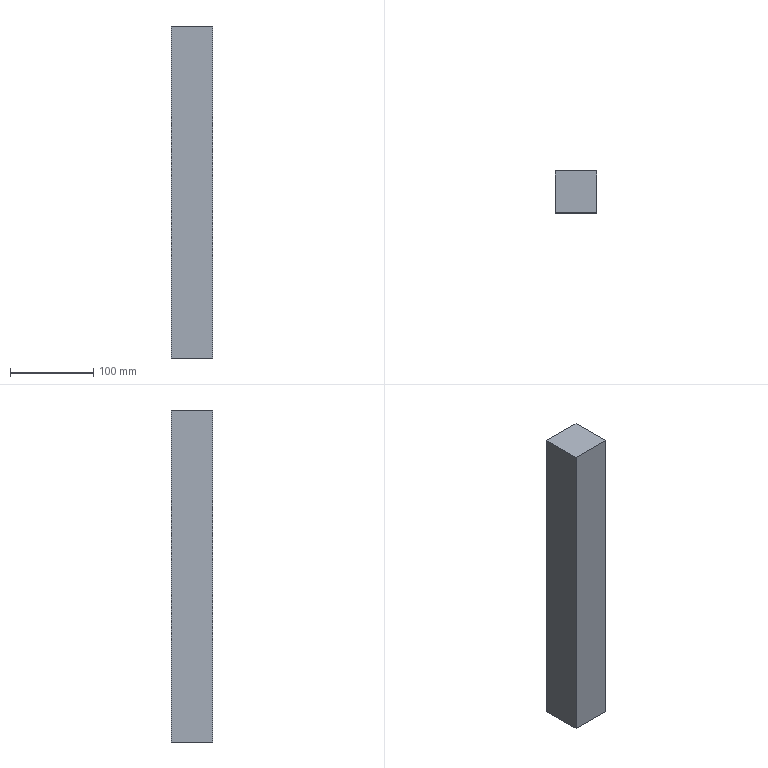Part | STEP file | 1 solid | 6 faces | box 50 x 50 x 400 mm | volume 1000000 mm3 | plane 6
STEP:
#1=CARTESIAN_POINT('',(0.,0.,0.));
#2=DIRECTION('',(0.,0.,1.));
#3=DIRECTION('',(1.,0.,0.));
#4=AXIS2_PLACEMENT_3D('',#1,#2,#3);
#5=CARTESIAN_POINT('',(-523.95,-190.836,-56.359));
#6=VERTEX_POINT('',#5);
#7=CARTESIAN_POINT('',(-473.95,-190.836,-56.359));
#8=VERTEX_POINT('',#7);
#9=CARTESIAN_POINT('',(-523.95,-190.836,-56.359));
#10=DIRECTION('',(1.,0.,0.));
#11=VECTOR('',#10,1.);
#12=LINE('',#9,#11);
#13=CARTESIAN_POINT('',(626.05,-190.836,-56.359));
#14=DIRECTION('',(0.,0.,1.));
#15=DIRECTION('',(1.,0.,0.));
#16=AXIS2_PLACEMENT_3D('',#13,#14,#15);
#17=PLANE('',#16);
#18=CARTESIAN_POINT('',(-1150.,0.));
#19=DIRECTION('',(1.,0.));
#20=VECTOR('',#19,1.);
#21=LINE('',#18,#20);
#22=(GEOMETRIC_REPRESENTATION_CONTEXT(2)PARAMETRIC_REPRESENTATION_CONTEXT()REPRESENTATION_CONTEXT('',''));
#23=DEFINITIONAL_REPRESENTATION('',(#21),#22);
#24=PCURVE('',#17,#23);
#25=CARTESIAN_POINT('',(-523.95,-190.836,203.641));
#26=DIRECTION('',(0.,1.,0.));
#27=DIRECTION('',(-1.,0.,0.));
#28=AXIS2_PLACEMENT_3D('',#25,#26,#27);
#29=PLANE('',#28);
#30=CARTESIAN_POINT('',(0.,-260.));
#31=DIRECTION('',(-1.,0.));
#32=VECTOR('',#31,1.);
#33=LINE('',#30,#32);
#34=(GEOMETRIC_REPRESENTATION_CONTEXT(2)PARAMETRIC_REPRESENTATION_CONTEXT()REPRESENTATION_CONTEXT('',''));
#35=DEFINITIONAL_REPRESENTATION('',(#33),#34);
#36=PCURVE('',#29,#35);
#37=SURFACE_CURVE('',#12,(#24,#36),.PCURVE_S1.);
#38=EDGE_CURVE('',#6,#8,#37,.T.);
#39=ORIENTED_EDGE('',*,*,#38,.T.);
#40=CARTESIAN_POINT('',(-473.95,-240.836,-56.359));
#41=VERTEX_POINT('',#40);
#42=CARTESIAN_POINT('',(-473.95,-1650.836,-56.359));
#43=DIRECTION('',(0.,1.,0.));
#44=VECTOR('',#43,1.);
#45=LINE('',#42,#44);
#46=CARTESIAN_POINT('',(-1100.,-1460.));
#47=DIRECTION('',(0.,1.));
#48=VECTOR('',#47,1.);
#49=LINE('',#46,#48);
#50=(GEOMETRIC_REPRESENTATION_CONTEXT(2)PARAMETRIC_REPRESENTATION_CONTEXT()REPRESENTATION_CONTEXT('',''));
#51=DEFINITIONAL_REPRESENTATION('',(#49),#50);
#52=PCURVE('',#17,#51);
#53=CARTESIAN_POINT('',(-473.95,-1650.836,-56.359));
#54=DIRECTION('',(-1.,0.,0.));
#55=DIRECTION('',(0.,-1.,0.));
#56=AXIS2_PLACEMENT_3D('',#53,#54,#55);
#57=PLANE('',#56);
#58=CARTESIAN_POINT('',(0.,0.));
#59=DIRECTION('',(-1.,0.));
#60=VECTOR('',#59,1.);
#61=LINE('',#58,#60);
#62=(GEOMETRIC_REPRESENTATION_CONTEXT(2)PARAMETRIC_REPRESENTATION_CONTEXT()REPRESENTATION_CONTEXT('',''));
#63=DEFINITIONAL_REPRESENTATION('',(#61),#62);
#64=PCURVE('',#57,#63);
#65=SURFACE_CURVE('',#45,(#52,#64),.PCURVE_S1.);
#66=EDGE_CURVE('',#41,#8,#65,.T.);
#67=ORIENTED_EDGE('',*,*,#66,.F.);
#68=CARTESIAN_POINT('',(-523.95,-240.836,-56.359));
#69=VERTEX_POINT('',#68);
#70=CARTESIAN_POINT('',(936.05,-240.836,-56.359));
#71=DIRECTION('',(-1.,0.,0.));
#72=VECTOR('',#71,1.);
#73=LINE('',#70,#72);
#74=CARTESIAN_POINT('',(310.,-50.));
#75=DIRECTION('',(-1.,0.));
#76=VECTOR('',#75,1.);
#77=LINE('',#74,#76);
#78=(GEOMETRIC_REPRESENTATION_CONTEXT(2)PARAMETRIC_REPRESENTATION_CONTEXT()REPRESENTATION_CONTEXT('',''));
#79=DEFINITIONAL_REPRESENTATION('',(#77),#78);
#80=PCURVE('',#17,#79);
#81=CARTESIAN_POINT('',(626.05,-240.836,-806.359));
#82=DIRECTION('',(0.,1.,0.));
#83=DIRECTION('',(-1.,0.,0.));
#84=AXIS2_PLACEMENT_3D('',#81,#82,#83);
#85=PLANE('',#84);
#86=CARTESIAN_POINT('',(-310.,750.));
#87=DIRECTION('',(1.,0.));
#88=VECTOR('',#87,1.);
#89=LINE('',#86,#88);
#90=(GEOMETRIC_REPRESENTATION_CONTEXT(2)PARAMETRIC_REPRESENTATION_CONTEXT()REPRESENTATION_CONTEXT('',''));
#91=DEFINITIONAL_REPRESENTATION('',(#89),#90);
#92=PCURVE('',#85,#91);
#93=SURFACE_CURVE('',#73,(#80,#92),.PCURVE_S1.);
#94=EDGE_CURVE('',#41,#69,#93,.T.);
#95=ORIENTED_EDGE('',*,*,#94,.T.);
#96=CARTESIAN_POINT('',(-523.95,0.,-56.359));
#97=DIRECTION('',(0.,-1.,0.));
#98=VECTOR('',#97,1.);
#99=LINE('',#96,#98);
#100=CARTESIAN_POINT('',(-1150.,190.836));
#101=DIRECTION('',(0.,-1.));
#102=VECTOR('',#101,1.);
#103=LINE('',#100,#102);
#104=(GEOMETRIC_REPRESENTATION_CONTEXT(2)PARAMETRIC_REPRESENTATION_CONTEXT()REPRESENTATION_CONTEXT('',''));
#105=DEFINITIONAL_REPRESENTATION('',(#103),#104);
#106=PCURVE('',#17,#105);
#107=CARTESIAN_POINT('',(-523.95,0.,203.641));
#108=DIRECTION('',(1.,0.,0.));
#109=DIRECTION('',(0.,0.,-1.));
#110=AXIS2_PLACEMENT_3D('',#107,#108,#109);
#111=PLANE('',#110);
#112=CARTESIAN_POINT('',(260.,0.));
#113=DIRECTION('',(0.,-1.));
#114=VECTOR('',#113,1.);
#115=LINE('',#112,#114);
#116=(GEOMETRIC_REPRESENTATION_CONTEXT(2)PARAMETRIC_REPRESENTATION_CONTEXT()REPRESENTATION_CONTEXT('',''));
#117=DEFINITIONAL_REPRESENTATION('',(#115),#116);
#118=PCURVE('',#111,#117);
#119=SURFACE_CURVE('',#99,(#106,#118),.PCURVE_S1.);
#120=EDGE_CURVE('',#6,#69,#119,.T.);
#121=ORIENTED_EDGE('',*,*,#120,.F.);
#122=EDGE_LOOP('',(#39,#67,#95,#121));
#123=FACE_BOUND('',#122,.T.);
#124=ADVANCED_FACE('',(#123),#17,.F.);
#125=CARTESIAN_POINT('',(-473.95,-240.836,343.641));
#126=VERTEX_POINT('',#125);
#127=CARTESIAN_POINT('',(-473.95,-190.836,343.641));
#128=VERTEX_POINT('',#127);
#129=CARTESIAN_POINT('',(-473.95,-1650.836,343.641));
#130=DIRECTION('',(0.,1.,0.));
#131=VECTOR('',#130,1.);
#132=LINE('',#129,#131);
#133=CARTESIAN_POINT('',(-473.95,-190.836,343.641));
#134=DIRECTION('',(0.,0.,-1.));
#135=DIRECTION('',(-1.,0.,0.));
#136=AXIS2_PLACEMENT_3D('',#133,#134,#135);
#137=PLANE('',#136);
#138=CARTESIAN_POINT('',(0.,-1460.));
#139=DIRECTION('',(0.,1.));
#140=VECTOR('',#139,1.);
#141=LINE('',#138,#140);
#142=(GEOMETRIC_REPRESENTATION_CONTEXT(2)PARAMETRIC_REPRESENTATION_CONTEXT()REPRESENTATION_CONTEXT('',''));
#143=DEFINITIONAL_REPRESENTATION('',(#141),#142);
#144=PCURVE('',#137,#143);
#145=CARTESIAN_POINT('',(0.,400.));
#146=DIRECTION('',(-1.,0.));
#147=VECTOR('',#146,1.);
#148=LINE('',#145,#147);
#149=(GEOMETRIC_REPRESENTATION_CONTEXT(2)PARAMETRIC_REPRESENTATION_CONTEXT()REPRESENTATION_CONTEXT('',''));
#150=DEFINITIONAL_REPRESENTATION('',(#148),#149);
#151=PCURVE('',#57,#150);
#152=SURFACE_CURVE('',#132,(#144,#151),.PCURVE_S1.);
#153=EDGE_CURVE('',#126,#128,#152,.T.);
#154=ORIENTED_EDGE('',*,*,#153,.T.);
#155=CARTESIAN_POINT('',(-523.95,-190.836,343.641));
#156=VERTEX_POINT('',#155);
#157=CARTESIAN_POINT('',(-523.95,-190.836,343.641));
#158=DIRECTION('',(-1.,0.,0.));
#159=VECTOR('',#158,1.);
#160=LINE('',#157,#159);
#161=CARTESIAN_POINT('',(50.,0.));
#162=DIRECTION('',(1.,0.));
#163=VECTOR('',#162,1.);
#164=LINE('',#161,#163);
#165=(GEOMETRIC_REPRESENTATION_CONTEXT(2)PARAMETRIC_REPRESENTATION_CONTEXT()REPRESENTATION_CONTEXT('',''));
#166=DEFINITIONAL_REPRESENTATION('',(#164),#165);
#167=PCURVE('',#137,#166);
#168=CARTESIAN_POINT('',(0.,140.));
#169=DIRECTION('',(1.,0.));
#170=VECTOR('',#169,1.);
#171=LINE('',#168,#170);
#172=(GEOMETRIC_REPRESENTATION_CONTEXT(2)PARAMETRIC_REPRESENTATION_CONTEXT()REPRESENTATION_CONTEXT('',''));
#173=DEFINITIONAL_REPRESENTATION('',(#171),#172);
#174=PCURVE('',#29,#173);
#175=SURFACE_CURVE('',#160,(#167,#174),.PCURVE_S1.);
#176=EDGE_CURVE('',#128,#156,#175,.T.);
#177=ORIENTED_EDGE('',*,*,#176,.T.);
#178=CARTESIAN_POINT('',(-523.95,-240.836,343.641));
#179=VERTEX_POINT('',#178);
#180=CARTESIAN_POINT('',(-523.95,0.,343.641));
#181=DIRECTION('',(0.,1.,0.));
#182=VECTOR('',#181,1.);
#183=LINE('',#180,#182);
#184=CARTESIAN_POINT('',(50.,190.836));
#185=DIRECTION('',(0.,1.));
#186=VECTOR('',#185,1.);
#187=LINE('',#184,#186);
#188=(GEOMETRIC_REPRESENTATION_CONTEXT(2)PARAMETRIC_REPRESENTATION_CONTEXT()REPRESENTATION_CONTEXT('',''));
#189=DEFINITIONAL_REPRESENTATION('',(#187),#188);
#190=PCURVE('',#137,#189);
#191=CARTESIAN_POINT('',(-140.,0.));
#192=DIRECTION('',(0.,1.));
#193=VECTOR('',#192,1.);
#194=LINE('',#191,#193);
#195=(GEOMETRIC_REPRESENTATION_CONTEXT(2)PARAMETRIC_REPRESENTATION_CONTEXT()REPRESENTATION_CONTEXT('',''));
#196=DEFINITIONAL_REPRESENTATION('',(#194),#195);
#197=PCURVE('',#111,#196);
#198=SURFACE_CURVE('',#183,(#190,#197),.PCURVE_S1.);
#199=EDGE_CURVE('',#179,#156,#198,.T.);
#200=ORIENTED_EDGE('',*,*,#199,.F.);
#201=CARTESIAN_POINT('',(936.05,-240.836,343.641));
#202=DIRECTION('',(-1.,0.,0.));
#203=VECTOR('',#202,1.);
#204=LINE('',#201,#203);
#205=CARTESIAN_POINT('',(-1410.,-50.));
#206=DIRECTION('',(1.,0.));
#207=VECTOR('',#206,1.);
#208=LINE('',#205,#207);
#209=(GEOMETRIC_REPRESENTATION_CONTEXT(2)PARAMETRIC_REPRESENTATION_CONTEXT()REPRESENTATION_CONTEXT('',''));
#210=DEFINITIONAL_REPRESENTATION('',(#208),#209);
#211=PCURVE('',#137,#210);
#212=CARTESIAN_POINT('',(-310.,1150.));
#213=DIRECTION('',(1.,0.));
#214=VECTOR('',#213,1.);
#215=LINE('',#212,#214);
#216=(GEOMETRIC_REPRESENTATION_CONTEXT(2)PARAMETRIC_REPRESENTATION_CONTEXT()REPRESENTATION_CONTEXT('',''));
#217=DEFINITIONAL_REPRESENTATION('',(#215),#216);
#218=PCURVE('',#85,#217);
#219=SURFACE_CURVE('',#204,(#211,#218),.PCURVE_S1.);
#220=EDGE_CURVE('',#126,#179,#219,.T.);
#221=ORIENTED_EDGE('',*,*,#220,.F.);
#222=EDGE_LOOP('',(#154,#177,#200,#221));
#223=FACE_BOUND('',#222,.T.);
#224=ADVANCED_FACE('',(#223),#137,.F.);
#225=ORIENTED_EDGE('',*,*,#66,.T.);
#226=CARTESIAN_POINT('',(-473.95,-190.836,-56.359));
#227=DIRECTION('',(0.,0.,1.));
#228=VECTOR('',#227,1.);
#229=LINE('',#226,#228);
#230=CARTESIAN_POINT('',(-1460.,0.));
#231=DIRECTION('',(0.,1.));
#232=VECTOR('',#231,1.);
#233=LINE('',#230,#232);
#234=(GEOMETRIC_REPRESENTATION_CONTEXT(2)PARAMETRIC_REPRESENTATION_CONTEXT()REPRESENTATION_CONTEXT('',''));
#235=DEFINITIONAL_REPRESENTATION('',(#233),#234);
#236=PCURVE('',#57,#235);
#237=CARTESIAN_POINT('',(-50.,-260.));
#238=DIRECTION('',(0.,1.));
#239=VECTOR('',#238,1.);
#240=LINE('',#237,#239);
#241=(GEOMETRIC_REPRESENTATION_CONTEXT(2)PARAMETRIC_REPRESENTATION_CONTEXT()REPRESENTATION_CONTEXT('',''));
#242=DEFINITIONAL_REPRESENTATION('',(#240),#241);
#243=PCURVE('',#29,#242);
#244=SURFACE_CURVE('',#229,(#236,#243),.PCURVE_S1.);
#245=EDGE_CURVE('',#8,#128,#244,.T.);
#246=ORIENTED_EDGE('',*,*,#245,.T.);
#247=ORIENTED_EDGE('',*,*,#153,.F.);
#248=CARTESIAN_POINT('',(-473.95,-240.836,-806.359));
#249=DIRECTION('',(0.,0.,1.));
#250=VECTOR('',#249,1.);
#251=LINE('',#248,#250);
#252=CARTESIAN_POINT('',(-1410.,-750.));
#253=DIRECTION('',(0.,1.));
#254=VECTOR('',#253,1.);
#255=LINE('',#252,#254);
#256=(GEOMETRIC_REPRESENTATION_CONTEXT(2)PARAMETRIC_REPRESENTATION_CONTEXT()REPRESENTATION_CONTEXT('',''));
#257=DEFINITIONAL_REPRESENTATION('',(#255),#256);
#258=PCURVE('',#57,#257);
#259=CARTESIAN_POINT('',(1100.,0.));
#260=DIRECTION('',(0.,1.));
#261=VECTOR('',#260,1.);
#262=LINE('',#259,#261);
#263=(GEOMETRIC_REPRESENTATION_CONTEXT(2)PARAMETRIC_REPRESENTATION_CONTEXT()REPRESENTATION_CONTEXT('',''));
#264=DEFINITIONAL_REPRESENTATION('',(#262),#263);
#265=PCURVE('',#85,#264);
#266=SURFACE_CURVE('',#251,(#258,#265),.PCURVE_S1.);
#267=EDGE_CURVE('',#41,#126,#266,.T.);
#268=ORIENTED_EDGE('',*,*,#267,.F.);
#269=EDGE_LOOP('',(#225,#246,#247,#268));
#270=FACE_BOUND('',#269,.T.);
#271=ADVANCED_FACE('',(#270),#57,.F.);
#272=ORIENTED_EDGE('',*,*,#38,.F.);
#273=CARTESIAN_POINT('',(-523.95,-190.836,393.641));
#274=DIRECTION('',(0.,0.,-1.));
#275=VECTOR('',#274,1.);
#276=LINE('',#273,#275);
#277=CARTESIAN_POINT('',(0.,190.));
#278=DIRECTION('',(0.,-1.));
#279=VECTOR('',#278,1.);
#280=LINE('',#277,#279);
#281=(GEOMETRIC_REPRESENTATION_CONTEXT(2)PARAMETRIC_REPRESENTATION_CONTEXT()REPRESENTATION_CONTEXT('',''));
#282=DEFINITIONAL_REPRESENTATION('',(#280),#281);
#283=PCURVE('',#29,#282);
#284=CARTESIAN_POINT('',(-190.,-190.836));
#285=DIRECTION('',(1.,0.));
#286=VECTOR('',#285,1.);
#287=LINE('',#284,#286);
#288=(GEOMETRIC_REPRESENTATION_CONTEXT(2)PARAMETRIC_REPRESENTATION_CONTEXT()REPRESENTATION_CONTEXT('',''));
#289=DEFINITIONAL_REPRESENTATION('',(#287),#288);
#290=PCURVE('',#111,#289);
#291=SURFACE_CURVE('',#276,(#283,#290),.PCURVE_S1.);
#292=EDGE_CURVE('',#156,#6,#291,.T.);
#293=ORIENTED_EDGE('',*,*,#292,.F.);
#294=ORIENTED_EDGE('',*,*,#176,.F.);
#295=ORIENTED_EDGE('',*,*,#245,.F.);
#296=EDGE_LOOP('',(#272,#293,#294,#295));
#297=FACE_BOUND('',#296,.T.);
#298=ADVANCED_FACE('',(#297),#29,.T.);
#299=ORIENTED_EDGE('',*,*,#94,.F.);
#300=ORIENTED_EDGE('',*,*,#267,.T.);
#301=ORIENTED_EDGE('',*,*,#220,.T.);
#302=CARTESIAN_POINT('',(-523.95,-240.836,343.641));
#303=DIRECTION('',(0.,0.,-1.));
#304=VECTOR('',#303,1.);
#305=LINE('',#302,#304);
#306=CARTESIAN_POINT('',(1150.,1150.));
#307=DIRECTION('',(0.,-1.));
#308=VECTOR('',#307,1.);
#309=LINE('',#306,#308);
#310=(GEOMETRIC_REPRESENTATION_CONTEXT(2)PARAMETRIC_REPRESENTATION_CONTEXT()REPRESENTATION_CONTEXT('',''));
#311=DEFINITIONAL_REPRESENTATION('',(#309),#310);
#312=PCURVE('',#85,#311);
#313=CARTESIAN_POINT('',(-140.,-240.836));
#314=DIRECTION('',(1.,0.));
#315=VECTOR('',#314,1.);
#316=LINE('',#313,#315);
#317=(GEOMETRIC_REPRESENTATION_CONTEXT(2)PARAMETRIC_REPRESENTATION_CONTEXT()REPRESENTATION_CONTEXT('',''));
#318=DEFINITIONAL_REPRESENTATION('',(#316),#317);
#319=PCURVE('',#111,#318);
#320=SURFACE_CURVE('',#305,(#312,#319),.PCURVE_S1.);
#321=EDGE_CURVE('',#179,#69,#320,.T.);
#322=ORIENTED_EDGE('',*,*,#321,.T.);
#323=EDGE_LOOP('',(#299,#300,#301,#322));
#324=FACE_BOUND('',#323,.T.);
#325=ADVANCED_FACE('',(#324),#85,.F.);
#326=ORIENTED_EDGE('',*,*,#292,.T.);
#327=ORIENTED_EDGE('',*,*,#120,.T.);
#328=ORIENTED_EDGE('',*,*,#321,.F.);
#329=ORIENTED_EDGE('',*,*,#199,.T.);
#330=EDGE_LOOP('',(#326,#327,#328,#329));
#331=FACE_BOUND('',#330,.T.);
#332=ADVANCED_FACE('',(#331),#111,.F.);
#333=CLOSED_SHELL('',(#124,#224,#271,#298,#325,#332));
#334=MANIFOLD_SOLID_BREP('',#333);
#335=(LENGTH_UNIT()NAMED_UNIT(*)SI_UNIT(.MILLI.,.METRE.));
#336=UNCERTAINTY_MEASURE_WITH_UNIT(LENGTH_MEASURE(0.0000001),#335,'','');
#337=(NAMED_UNIT(*)PLANE_ANGLE_UNIT()SI_UNIT($,.RADIAN.));
#338=(NAMED_UNIT(*)SI_UNIT($,.STERADIAN.)SOLID_ANGLE_UNIT());
#339=(GEOMETRIC_REPRESENTATION_CONTEXT(3)GLOBAL_UNCERTAINTY_ASSIGNED_CONTEXT((#336))GLOBAL_UNIT_ASSIGNED_CONTEXT((#335,#337,#338))REPRESENTATION_CONTEXT('',''));
#340=ADVANCED_BREP_SHAPE_REPRESENTATION('',(#4,#334),#339);